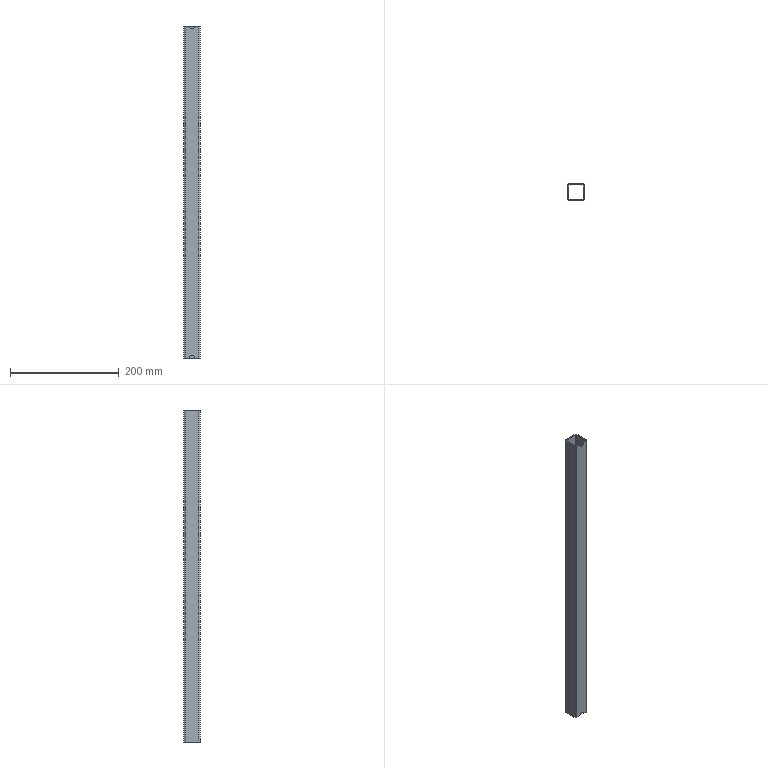Part | STEP file | PN_0030_default | 1 solid | 20 faces | box 30 x 30 x 612 mm | volume 101776 mm3 | plane 10 | cylinder 10 | commonest cylinder face diameters 2 x4 5 x4 10 x2